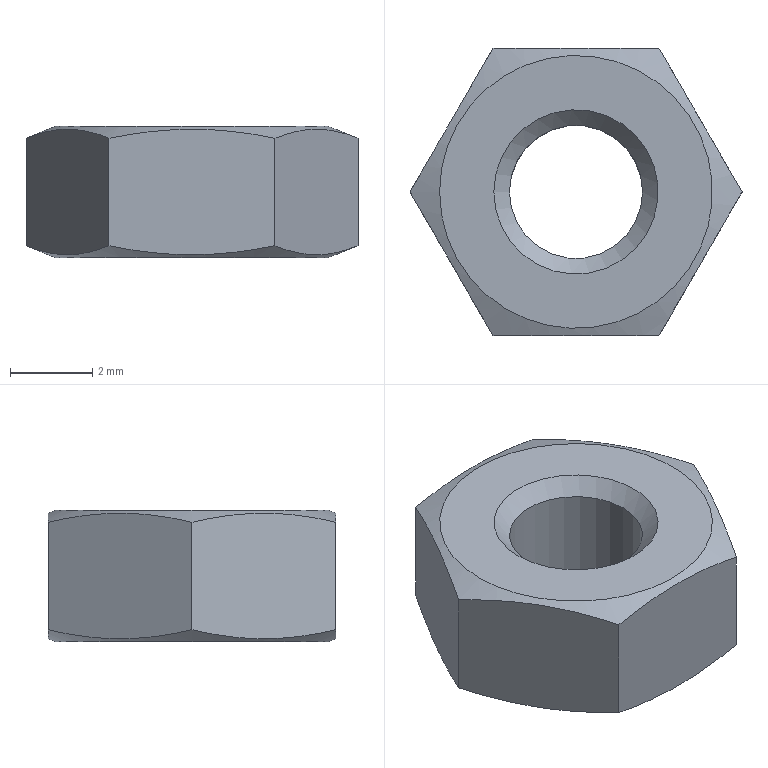Part | STEP file | 1_33 | 1 solid | 13 faces | box 8.083 x 7 x 3.2 mm | volume 106.427 mm3 | plane 8 | cone 4 | cylinder 1 | commonest cylinder face diameters 3.242 x1
STEP:
#1=CARTESIAN_POINT('',(0.,0.,0.));
#2=DIRECTION('',(0.,0.,1.));
#3=DIRECTION('',(1.,0.,0.));
#4=AXIS2_PLACEMENT_3D('',#1,#2,#3);
#5=CARTESIAN_POINT('',(-1.621,0.,0.3789));
#6=VERTEX_POINT('',#5);
#7=CARTESIAN_POINT('',(0.,0.,0.3789));
#8=DIRECTION('',(0.,0.,-1.));
#9=DIRECTION('',(1.,0.,0.));
#10=AXIS2_PLACEMENT_3D('',#7,#8,#9);
#11=CIRCLE('',#10,1.621);
#12=CARTESIAN_POINT('',(0.,0.,0.1894));
#13=DIRECTION('',(0.,0.,-1.));
#14=DIRECTION('',(1.,0.,0.));
#15=AXIS2_PLACEMENT_3D('',#12,#13,#14);
#16=CONICAL_SURFACE('',#15,1.811,0.7854);
#17=CARTESIAN_POINT('',(0.,-0.1894));
#18=DIRECTION('',(1.,0.));
#19=VECTOR('',#18,1.);
#20=LINE('',#17,#19);
#21=(GEOMETRIC_REPRESENTATION_CONTEXT(2)PARAMETRIC_REPRESENTATION_CONTEXT()REPRESENTATION_CONTEXT('',''));
#22=DEFINITIONAL_REPRESENTATION('',(#20),#21);
#23=PCURVE('',#16,#22);
#24=CARTESIAN_POINT('',(0.,0.,1.6));
#25=DIRECTION('',(0.,0.,-1.));
#26=DIRECTION('',(1.,0.,0.));
#27=AXIS2_PLACEMENT_3D('',#24,#25,#26);
#28=CYLINDRICAL_SURFACE('',#27,1.621);
#29=CARTESIAN_POINT('',(0.,1.221));
#30=DIRECTION('',(1.,0.));
#31=VECTOR('',#30,1.);
#32=LINE('',#29,#31);
#33=(GEOMETRIC_REPRESENTATION_CONTEXT(2)PARAMETRIC_REPRESENTATION_CONTEXT()REPRESENTATION_CONTEXT('',''));
#34=DEFINITIONAL_REPRESENTATION('',(#32),#33);
#35=PCURVE('',#28,#34);
#36=SURFACE_CURVE('',#11,(#23,#35),.PCURVE_S1.);
#37=EDGE_CURVE('',#6,#6,#36,.T.);
#38=ORIENTED_EDGE('',*,*,#37,.T.);
#39=CARTESIAN_POINT('',(-2.,0.,0.));
#40=VERTEX_POINT('',#39);
#41=CARTESIAN_POINT('',(-1.621,0.,0.3789));
#42=CARTESIAN_POINT('',(-2.,0.,0.));
#43=B_SPLINE_CURVE_WITH_KNOTS('',1,(#41,#42),.UNSPECIFIED.,.F.,.F.,(2,2),(-0.2679,0.2679),.PIECEWISE_BEZIER_KNOTS.);
#44=CARTESIAN_POINT('',(9.425,0.));
#45=DIRECTION('',(0.,1.));
#46=VECTOR('',#45,1.);
#47=LINE('',#44,#46);
#48=(GEOMETRIC_REPRESENTATION_CONTEXT(2)PARAMETRIC_REPRESENTATION_CONTEXT()REPRESENTATION_CONTEXT('',''));
#49=DEFINITIONAL_REPRESENTATION('',(#47),#48);
#50=PCURVE('',#16,#49);
#51=CARTESIAN_POINT('',(3.142,0.));
#52=DIRECTION('',(0.,1.));
#53=VECTOR('',#52,1.);
#54=LINE('',#51,#53);
#55=(GEOMETRIC_REPRESENTATION_CONTEXT(2)PARAMETRIC_REPRESENTATION_CONTEXT()REPRESENTATION_CONTEXT('',''));
#56=DEFINITIONAL_REPRESENTATION('',(#54),#55);
#57=PCURVE('',#16,#56);
#58=SEAM_CURVE('',#43,(#50,#57),.PCURVE_S1.);
#59=EDGE_CURVE('',#6,#40,#58,.T.);
#60=ORIENTED_EDGE('',*,*,#59,.T.);
#61=CARTESIAN_POINT('',(0.,0.,0.));
#62=DIRECTION('',(0.,0.,-1.));
#63=DIRECTION('',(1.,0.,0.));
#64=AXIS2_PLACEMENT_3D('',#61,#62,#63);
#65=CIRCLE('',#64,2.);
#66=CARTESIAN_POINT('',(0.,0.1894));
#67=DIRECTION('',(1.,0.));
#68=VECTOR('',#67,1.);
#69=LINE('',#66,#68);
#70=(GEOMETRIC_REPRESENTATION_CONTEXT(2)PARAMETRIC_REPRESENTATION_CONTEXT()REPRESENTATION_CONTEXT('',''));
#71=DEFINITIONAL_REPRESENTATION('',(#69),#70);
#72=PCURVE('',#16,#71);
#73=CARTESIAN_POINT('',(0.,0.,0.));
#74=DIRECTION('',(0.,0.,1.));
#75=DIRECTION('',(1.,0.,0.));
#76=AXIS2_PLACEMENT_3D('',#73,#74,#75);
#77=PLANE('',#76);
#78=CARTESIAN_POINT('',(2.,0.));
#79=CARTESIAN_POINT('',(2.,-3.464));
#80=CARTESIAN_POINT('',(-1.,-1.732));
#81=CARTESIAN_POINT('',(-4.,0.));
#82=CARTESIAN_POINT('',(-1.,1.732));
#83=CARTESIAN_POINT('',(2.,3.464));
#84=CARTESIAN_POINT('',(2.,0.));
#85=(BOUNDED_CURVE()B_SPLINE_CURVE(2,(#78,#79,#80,#81,#82,#83,#84),.UNSPECIFIED.,.T.,.F.)B_SPLINE_CURVE_WITH_KNOTS((1,2,2,2,2,1),(-2.094,0.,2.094,4.189,6.283,8.378),.UNSPECIFIED.)CURVE()GEOMETRIC_REPRESENTATION_ITEM()RATIONAL_B_SPLINE_CURVE((1.,0.5,1.,0.5,1.,0.5,1.))REPRESENTATION_ITEM(''));
#86=(GEOMETRIC_REPRESENTATION_CONTEXT(2)PARAMETRIC_REPRESENTATION_CONTEXT()REPRESENTATION_CONTEXT('',''));
#87=DEFINITIONAL_REPRESENTATION('',(#85),#86);
#88=PCURVE('',#77,#87);
#89=SURFACE_CURVE('',#65,(#72,#88),.PCURVE_S1.);
#90=EDGE_CURVE('',#40,#40,#89,.T.);
#91=ORIENTED_EDGE('',*,*,#90,.F.);
#92=ORIENTED_EDGE('',*,*,#59,.F.);
#93=EDGE_LOOP('',(#38,#60,#91,#92));
#94=FACE_BOUND('',#93,.F.);
#95=ADVANCED_FACE('',(#94),#16,.F.);
#96=CARTESIAN_POINT('',(-3.321,0.,0.));
#97=VERTEX_POINT('',#96);
#98=CARTESIAN_POINT('',(0.,0.,0.));
#99=DIRECTION('',(0.,0.,1.));
#100=DIRECTION('',(1.,0.,0.));
#101=AXIS2_PLACEMENT_3D('',#98,#99,#100);
#102=CIRCLE('',#101,3.321);
#103=CARTESIAN_POINT('',(0.,0.));
#104=DIRECTION('',(1.,0.));
#105=AXIS2_PLACEMENT_2D('',#103,#104);
#106=CIRCLE('',#105,3.321);
#107=(GEOMETRIC_REPRESENTATION_CONTEXT(2)PARAMETRIC_REPRESENTATION_CONTEXT()REPRESENTATION_CONTEXT('',''));
#108=DEFINITIONAL_REPRESENTATION('',(#106),#107);
#109=PCURVE('',#77,#108);
#110=CARTESIAN_POINT('',(0.,0.,0.1455));
#111=DIRECTION('',(0.,0.,1.));
#112=DIRECTION('',(1.,0.,0.));
#113=AXIS2_PLACEMENT_3D('',#110,#111,#112);
#114=CONICAL_SURFACE('',#113,3.681,1.187);
#115=CARTESIAN_POINT('',(0.,-0.1455));
#116=DIRECTION('',(1.,0.));
#117=VECTOR('',#116,1.);
#118=LINE('',#115,#117);
#119=(GEOMETRIC_REPRESENTATION_CONTEXT(2)PARAMETRIC_REPRESENTATION_CONTEXT()REPRESENTATION_CONTEXT('',''));
#120=DEFINITIONAL_REPRESENTATION('',(#118),#119);
#121=PCURVE('',#114,#120);
#122=SURFACE_CURVE('',#102,(#109,#121),.PCURVE_S1.);
#123=EDGE_CURVE('',#97,#97,#122,.T.);
#124=ORIENTED_EDGE('',*,*,#123,.F.);
#125=EDGE_LOOP('',(#124));
#126=FACE_BOUND('',#125,.T.);
#127=ORIENTED_EDGE('',*,*,#90,.F.);
#128=EDGE_LOOP('',(#127));
#129=FACE_BOUND('',#128,.T.);
#130=ADVANCED_FACE('',(#126,#129),#77,.F.);
#131=CARTESIAN_POINT('',(-1.621,0.,2.821));
#132=VERTEX_POINT('',#131);
#133=CARTESIAN_POINT('',(0.,0.,2.821));
#134=DIRECTION('',(0.,0.,-1.));
#135=DIRECTION('',(1.,0.,0.));
#136=AXIS2_PLACEMENT_3D('',#133,#134,#135);
#137=CIRCLE('',#136,1.621);
#138=CARTESIAN_POINT('',(0.,-1.221));
#139=DIRECTION('',(1.,0.));
#140=VECTOR('',#139,1.);
#141=LINE('',#138,#140);
#142=(GEOMETRIC_REPRESENTATION_CONTEXT(2)PARAMETRIC_REPRESENTATION_CONTEXT()REPRESENTATION_CONTEXT('',''));
#143=DEFINITIONAL_REPRESENTATION('',(#141),#142);
#144=PCURVE('',#28,#143);
#145=CARTESIAN_POINT('',(0.,0.,3.011));
#146=DIRECTION('',(0.,0.,1.));
#147=DIRECTION('',(-1.,0.,0.));
#148=AXIS2_PLACEMENT_3D('',#145,#146,#147);
#149=CONICAL_SURFACE('',#148,1.811,0.7854);
#150=CARTESIAN_POINT('',(9.425,-0.1894));
#151=DIRECTION('',(-1.,0.));
#152=VECTOR('',#151,1.);
#153=LINE('',#150,#152);
#154=(GEOMETRIC_REPRESENTATION_CONTEXT(2)PARAMETRIC_REPRESENTATION_CONTEXT()REPRESENTATION_CONTEXT('',''));
#155=DEFINITIONAL_REPRESENTATION('',(#153),#154);
#156=PCURVE('',#149,#155);
#157=SURFACE_CURVE('',#137,(#144,#156),.PCURVE_S1.);
#158=EDGE_CURVE('',#132,#132,#157,.T.);
#159=ORIENTED_EDGE('',*,*,#158,.T.);
#160=CARTESIAN_POINT('',(-1.621,0.,2.821));
#161=CARTESIAN_POINT('',(-1.621,0.,0.3789));
#162=B_SPLINE_CURVE_WITH_KNOTS('',1,(#160,#161),.UNSPECIFIED.,.F.,.F.,(2,2),(-1.221,1.221),.PIECEWISE_BEZIER_KNOTS.);
#163=CARTESIAN_POINT('',(9.425,0.));
#164=DIRECTION('',(0.,1.));
#165=VECTOR('',#164,1.);
#166=LINE('',#163,#165);
#167=(GEOMETRIC_REPRESENTATION_CONTEXT(2)PARAMETRIC_REPRESENTATION_CONTEXT()REPRESENTATION_CONTEXT('',''));
#168=DEFINITIONAL_REPRESENTATION('',(#166),#167);
#169=PCURVE('',#28,#168);
#170=CARTESIAN_POINT('',(3.142,0.));
#171=DIRECTION('',(0.,1.));
#172=VECTOR('',#171,1.);
#173=LINE('',#170,#172);
#174=(GEOMETRIC_REPRESENTATION_CONTEXT(2)PARAMETRIC_REPRESENTATION_CONTEXT()REPRESENTATION_CONTEXT('',''));
#175=DEFINITIONAL_REPRESENTATION('',(#173),#174);
#176=PCURVE('',#28,#175);
#177=SEAM_CURVE('',#162,(#169,#176),.PCURVE_S1.);
#178=EDGE_CURVE('',#132,#6,#177,.T.);
#179=ORIENTED_EDGE('',*,*,#178,.T.);
#180=ORIENTED_EDGE('',*,*,#37,.F.);
#181=ORIENTED_EDGE('',*,*,#178,.F.);
#182=EDGE_LOOP('',(#159,#179,#180,#181));
#183=FACE_BOUND('',#182,.F.);
#184=ADVANCED_FACE('',(#183),#28,.F.);
#185=CARTESIAN_POINT('',(-4.041,0.,0.2909));
#186=VERTEX_POINT('',#185);
#187=CARTESIAN_POINT('',(-2.021,3.5,0.2909));
#188=VERTEX_POINT('',#187);
#189=CARTESIAN_POINT('',(-9.627,-9.674,4.172));
#190=CARTESIAN_POINT('',(-3.031,1.75,-0.9793));
#191=CARTESIAN_POINT('',(3.564,13.174,4.172));
#192=(BOUNDED_CURVE()B_SPLINE_CURVE(2,(#189,#190,#191),.UNSPECIFIED.,.F.,.F.)B_SPLINE_CURVE_WITH_KNOTS((3,3),(0.,2.763),.PIECEWISE_BEZIER_KNOTS.)CURVE()GEOMETRIC_REPRESENTATION_ITEM()RATIONAL_B_SPLINE_CURVE((1.,3.899,1.))REPRESENTATION_ITEM(''));
#193=CARTESIAN_POINT('',(9.425,0.1455));
#194=CARTESIAN_POINT('',(9.41,0.1312));
#195=CARTESIAN_POINT('',(9.379,0.1043));
#196=CARTESIAN_POINT('',(9.333,0.06874));
#197=CARTESIAN_POINT('',(9.286,0.03763));
#198=CARTESIAN_POINT('',(9.239,0.01072));
#199=CARTESIAN_POINT('',(9.191,-0.01221));
#200=CARTESIAN_POINT('',(9.144,-0.03133));
#201=CARTESIAN_POINT('',(9.095,-0.04679));
#202=CARTESIAN_POINT('',(9.047,-0.0587));
#203=CARTESIAN_POINT('',(8.999,-0.06714));
#204=CARTESIAN_POINT('',(8.95,-0.07219));
#205=CARTESIAN_POINT('',(8.901,-0.07387));
#206=CARTESIAN_POINT('',(8.852,-0.07219));
#207=CARTESIAN_POINT('',(8.804,-0.06714));
#208=CARTESIAN_POINT('',(8.755,-0.0587));
#209=CARTESIAN_POINT('',(8.707,-0.04679));
#210=CARTESIAN_POINT('',(8.659,-0.03133));
#211=CARTESIAN_POINT('',(8.611,-0.01221));
#212=CARTESIAN_POINT('',(8.563,0.01072));
#213=CARTESIAN_POINT('',(8.516,0.03763));
#214=CARTESIAN_POINT('',(8.469,0.06874));
#215=CARTESIAN_POINT('',(8.423,0.1043));
#216=CARTESIAN_POINT('',(8.393,0.1312));
#217=CARTESIAN_POINT('',(8.378,0.1455));
#218=B_SPLINE_CURVE_WITH_KNOTS('',3,(#193,#194,#195,#196,#197,#198,#199,#200,#201,#202,#203,#204,#205,#206,#207,#208,#209,#210,#211,#212,#213,#214,#215,#216,#217),.UNSPECIFIED.,.F.,.F.,(4,1,1,1,1,1,1,1,1,1,1,1,1,1,1,1,1,1,1,1,1,1,4),(0.9002,0.9439,0.9877,1.031,1.075,1.119,1.163,1.206,1.25,1.294,1.338,1.381,1.425,1.469,1.513,1.556,1.6,1.644,1.688,1.731,1.775,1.819,1.863),.QUASI_UNIFORM_KNOTS.);
#219=(GEOMETRIC_REPRESENTATION_CONTEXT(2)PARAMETRIC_REPRESENTATION_CONTEXT()REPRESENTATION_CONTEXT('',''));
#220=DEFINITIONAL_REPRESENTATION('',(#218),#219);
#221=PCURVE('',#114,#220);
#222=CARTESIAN_POINT('',(-4.041,0.,0.));
#223=DIRECTION('',(-0.866,0.5,0.));
#224=DIRECTION('',(0.,0.,1.));
#225=AXIS2_PLACEMENT_3D('',#222,#223,#224);
#226=PLANE('',#225);
#227=CARTESIAN_POINT('',(4.172,-11.17));
#228=CARTESIAN_POINT('',(-0.9793,2.021));
#229=CARTESIAN_POINT('',(4.172,15.212));
#230=(BOUNDED_CURVE()B_SPLINE_CURVE(2,(#227,#228,#229),.UNSPECIFIED.,.F.,.F.)B_SPLINE_CURVE_WITH_KNOTS((3,3),(0.,2.763),.PIECEWISE_BEZIER_KNOTS.)CURVE()GEOMETRIC_REPRESENTATION_ITEM()RATIONAL_B_SPLINE_CURVE((1.,3.899,1.))REPRESENTATION_ITEM(''));
#231=(GEOMETRIC_REPRESENTATION_CONTEXT(2)PARAMETRIC_REPRESENTATION_CONTEXT()REPRESENTATION_CONTEXT('',''));
#232=DEFINITIONAL_REPRESENTATION('',(#230),#231);
#233=PCURVE('',#226,#232);
#234=SURFACE_CURVE('',#192,(#221,#233),.PCURVE_S1.);
#235=EDGE_CURVE('',#186,#188,#234,.T.);
#236=ORIENTED_EDGE('',*,*,#235,.T.);
#237=CARTESIAN_POINT('',(2.021,3.5,0.2909));
#238=VERTEX_POINT('',#237);
#239=CARTESIAN_POINT('',(-13.191,3.5,4.172));
#240=CARTESIAN_POINT('',(0.,3.5,-0.9793));
#241=CARTESIAN_POINT('',(13.191,3.5,4.172));
#242=(BOUNDED_CURVE()B_SPLINE_CURVE(2,(#239,#240,#241),.UNSPECIFIED.,.F.,.F.)B_SPLINE_CURVE_WITH_KNOTS((3,3),(0.,2.763),.PIECEWISE_BEZIER_KNOTS.)CURVE()GEOMETRIC_REPRESENTATION_ITEM()RATIONAL_B_SPLINE_CURVE((1.,3.899,1.))REPRESENTATION_ITEM(''));
#243=CARTESIAN_POINT('',(8.378,0.1455));
#244=CARTESIAN_POINT('',(8.362,0.1312));
#245=CARTESIAN_POINT('',(8.332,0.1043));
#246=CARTESIAN_POINT('',(8.286,0.06874));
#247=CARTESIAN_POINT('',(8.239,0.03763));
#248=CARTESIAN_POINT('',(8.192,0.01072));
#249=CARTESIAN_POINT('',(8.144,-0.01221));
#250=CARTESIAN_POINT('',(8.096,-0.03133));
#251=CARTESIAN_POINT('',(8.048,-0.04679));
#252=CARTESIAN_POINT('',(8.,-0.0587));
#253=CARTESIAN_POINT('',(7.951,-0.06714));
#254=CARTESIAN_POINT('',(7.903,-0.07219));
#255=CARTESIAN_POINT('',(7.854,-0.07387));
#256=CARTESIAN_POINT('',(7.805,-0.07219));
#257=CARTESIAN_POINT('',(7.757,-0.06714));
#258=CARTESIAN_POINT('',(7.708,-0.0587));
#259=CARTESIAN_POINT('',(7.66,-0.04679));
#260=CARTESIAN_POINT('',(7.612,-0.03133));
#261=CARTESIAN_POINT('',(7.564,-0.01221));
#262=CARTESIAN_POINT('',(7.516,0.01072));
#263=CARTESIAN_POINT('',(7.469,0.03763));
#264=CARTESIAN_POINT('',(7.422,0.06874));
#265=CARTESIAN_POINT('',(7.376,0.1043));
#266=CARTESIAN_POINT('',(7.346,0.1312));
#267=CARTESIAN_POINT('',(7.33,0.1455));
#268=B_SPLINE_CURVE_WITH_KNOTS('',3,(#243,#244,#245,#246,#247,#248,#249,#250,#251,#252,#253,#254,#255,#256,#257,#258,#259,#260,#261,#262,#263,#264,#265,#266,#267),.UNSPECIFIED.,.F.,.F.,(4,1,1,1,1,1,1,1,1,1,1,1,1,1,1,1,1,1,1,1,1,1,4),(0.9002,0.9439,0.9877,1.031,1.075,1.119,1.163,1.206,1.25,1.294,1.338,1.381,1.425,1.469,1.513,1.556,1.6,1.644,1.688,1.731,1.775,1.819,1.863),.QUASI_UNIFORM_KNOTS.);
#269=(GEOMETRIC_REPRESENTATION_CONTEXT(2)PARAMETRIC_REPRESENTATION_CONTEXT()REPRESENTATION_CONTEXT('',''));
#270=DEFINITIONAL_REPRESENTATION('',(#268),#269);
#271=PCURVE('',#114,#270);
#272=CARTESIAN_POINT('',(-2.021,3.5,0.));
#273=DIRECTION('',(0.,1.,0.));
#274=DIRECTION('',(0.,0.,1.));
#275=AXIS2_PLACEMENT_3D('',#272,#273,#274);
#276=PLANE('',#275);
#277=CARTESIAN_POINT('',(4.172,-11.17));
#278=CARTESIAN_POINT('',(-0.9793,2.021));
#279=CARTESIAN_POINT('',(4.172,15.212));
#280=(BOUNDED_CURVE()B_SPLINE_CURVE(2,(#277,#278,#279),.UNSPECIFIED.,.F.,.F.)B_SPLINE_CURVE_WITH_KNOTS((3,3),(0.,2.763),.PIECEWISE_BEZIER_KNOTS.)CURVE()GEOMETRIC_REPRESENTATION_ITEM()RATIONAL_B_SPLINE_CURVE((1.,3.899,1.))REPRESENTATION_ITEM(''));
#281=(GEOMETRIC_REPRESENTATION_CONTEXT(2)PARAMETRIC_REPRESENTATION_CONTEXT()REPRESENTATION_CONTEXT('',''));
#282=DEFINITIONAL_REPRESENTATION('',(#280),#281);
#283=PCURVE('',#276,#282);
#284=SURFACE_CURVE('',#242,(#271,#283),.PCURVE_S1.);
#285=EDGE_CURVE('',#188,#238,#284,.T.);
#286=ORIENTED_EDGE('',*,*,#285,.T.);
#287=CARTESIAN_POINT('',(4.041,0.,0.2909));
#288=VERTEX_POINT('',#287);
#289=CARTESIAN_POINT('',(-3.564,13.174,4.172));
#290=CARTESIAN_POINT('',(3.031,1.75,-0.9793));
#291=CARTESIAN_POINT('',(9.627,-9.674,4.172));
#292=(BOUNDED_CURVE()B_SPLINE_CURVE(2,(#289,#290,#291),.UNSPECIFIED.,.F.,.F.)B_SPLINE_CURVE_WITH_KNOTS((3,3),(0.,2.763),.PIECEWISE_BEZIER_KNOTS.)CURVE()GEOMETRIC_REPRESENTATION_ITEM()RATIONAL_B_SPLINE_CURVE((1.,3.899,1.))REPRESENTATION_ITEM(''));
#293=CARTESIAN_POINT('',(7.33,0.1455));
#294=CARTESIAN_POINT('',(7.315,0.1312));
#295=CARTESIAN_POINT('',(7.285,0.1043));
#296=CARTESIAN_POINT('',(7.238,0.06874));
#297=CARTESIAN_POINT('',(7.192,0.03763));
#298=CARTESIAN_POINT('',(7.145,0.01072));
#299=CARTESIAN_POINT('',(7.097,-0.01221));
#300=CARTESIAN_POINT('',(7.049,-0.03133));
#301=CARTESIAN_POINT('',(7.001,-0.04679));
#302=CARTESIAN_POINT('',(6.953,-0.0587));
#303=CARTESIAN_POINT('',(6.904,-0.06714));
#304=CARTESIAN_POINT('',(6.856,-0.07219));
#305=CARTESIAN_POINT('',(6.807,-0.07387));
#306=CARTESIAN_POINT('',(6.758,-0.07219));
#307=CARTESIAN_POINT('',(6.709,-0.06714));
#308=CARTESIAN_POINT('',(6.661,-0.0587));
#309=CARTESIAN_POINT('',(6.612,-0.04679));
#310=CARTESIAN_POINT('',(6.564,-0.03133));
#311=CARTESIAN_POINT('',(6.516,-0.01221));
#312=CARTESIAN_POINT('',(6.469,0.01072));
#313=CARTESIAN_POINT('',(6.422,0.03763));
#314=CARTESIAN_POINT('',(6.375,0.06874));
#315=CARTESIAN_POINT('',(6.329,0.1043));
#316=CARTESIAN_POINT('',(6.298,0.1312));
#317=CARTESIAN_POINT('',(6.283,0.1455));
#318=B_SPLINE_CURVE_WITH_KNOTS('',3,(#293,#294,#295,#296,#297,#298,#299,#300,#301,#302,#303,#304,#305,#306,#307,#308,#309,#310,#311,#312,#313,#314,#315,#316,#317),.UNSPECIFIED.,.F.,.F.,(4,1,1,1,1,1,1,1,1,1,1,1,1,1,1,1,1,1,1,1,1,1,4),(0.9002,0.9439,0.9877,1.031,1.075,1.119,1.163,1.206,1.25,1.294,1.338,1.381,1.425,1.469,1.513,1.556,1.6,1.644,1.688,1.731,1.775,1.819,1.863),.QUASI_UNIFORM_KNOTS.);
#319=(GEOMETRIC_REPRESENTATION_CONTEXT(2)PARAMETRIC_REPRESENTATION_CONTEXT()REPRESENTATION_CONTEXT('',''));
#320=DEFINITIONAL_REPRESENTATION('',(#318),#319);
#321=PCURVE('',#114,#320);
#322=CARTESIAN_POINT('',(2.021,3.5,0.));
#323=DIRECTION('',(0.866,0.5,0.));
#324=DIRECTION('',(0.,0.,-1.));
#325=AXIS2_PLACEMENT_3D('',#322,#323,#324);
#326=PLANE('',#325);
#327=CARTESIAN_POINT('',(-4.172,11.17));
#328=CARTESIAN_POINT('',(0.9793,-2.021));
#329=CARTESIAN_POINT('',(-4.172,-15.212));
#330=(BOUNDED_CURVE()B_SPLINE_CURVE(2,(#327,#328,#329),.UNSPECIFIED.,.F.,.F.)B_SPLINE_CURVE_WITH_KNOTS((3,3),(0.,2.763),.PIECEWISE_BEZIER_KNOTS.)CURVE()GEOMETRIC_REPRESENTATION_ITEM()RATIONAL_B_SPLINE_CURVE((1.,3.899,1.))REPRESENTATION_ITEM(''));
#331=(GEOMETRIC_REPRESENTATION_CONTEXT(2)PARAMETRIC_REPRESENTATION_CONTEXT()REPRESENTATION_CONTEXT('',''));
#332=DEFINITIONAL_REPRESENTATION('',(#330),#331);
#333=PCURVE('',#326,#332);
#334=SURFACE_CURVE('',#292,(#321,#333),.PCURVE_S1.);
#335=EDGE_CURVE('',#238,#288,#334,.T.);
#336=ORIENTED_EDGE('',*,*,#335,.T.);
#337=CARTESIAN_POINT('',(2.021,-3.5,0.2909));
#338=VERTEX_POINT('',#337);
#339=CARTESIAN_POINT('',(9.627,9.674,4.172));
#340=CARTESIAN_POINT('',(3.031,-1.75,-0.9793));
#341=CARTESIAN_POINT('',(-3.564,-13.174,4.172));
#342=(BOUNDED_CURVE()B_SPLINE_CURVE(2,(#339,#340,#341),.UNSPECIFIED.,.F.,.F.)B_SPLINE_CURVE_WITH_KNOTS((3,3),(0.,2.763),.PIECEWISE_BEZIER_KNOTS.)CURVE()GEOMETRIC_REPRESENTATION_ITEM()RATIONAL_B_SPLINE_CURVE((1.,3.899,1.))REPRESENTATION_ITEM(''));
#343=CARTESIAN_POINT('',(6.283,0.1455));
#344=CARTESIAN_POINT('',(6.268,0.1312));
#345=CARTESIAN_POINT('',(6.238,0.1043));
#346=CARTESIAN_POINT('',(6.191,0.06874));
#347=CARTESIAN_POINT('',(6.145,0.03763));
#348=CARTESIAN_POINT('',(6.097,0.01072));
#349=CARTESIAN_POINT('',(6.05,-0.01221));
#350=CARTESIAN_POINT('',(6.002,-0.03133));
#351=CARTESIAN_POINT('',(5.954,-0.04679));
#352=CARTESIAN_POINT('',(5.906,-0.0587));
#353=CARTESIAN_POINT('',(5.857,-0.06714));
#354=CARTESIAN_POINT('',(5.808,-0.07219));
#355=CARTESIAN_POINT('',(5.76,-0.07387));
#356=CARTESIAN_POINT('',(5.711,-0.07219));
#357=CARTESIAN_POINT('',(5.662,-0.06714));
#358=CARTESIAN_POINT('',(5.614,-0.0587));
#359=CARTESIAN_POINT('',(5.565,-0.04679));
#360=CARTESIAN_POINT('',(5.517,-0.03133));
#361=CARTESIAN_POINT('',(5.469,-0.01221));
#362=CARTESIAN_POINT('',(5.422,0.01072));
#363=CARTESIAN_POINT('',(5.375,0.03763));
#364=CARTESIAN_POINT('',(5.328,0.06874));
#365=CARTESIAN_POINT('',(5.282,0.1043));
#366=CARTESIAN_POINT('',(5.251,0.1312));
#367=CARTESIAN_POINT('',(5.236,0.1455));
#368=B_SPLINE_CURVE_WITH_KNOTS('',3,(#343,#344,#345,#346,#347,#348,#349,#350,#351,#352,#353,#354,#355,#356,#357,#358,#359,#360,#361,#362,#363,#364,#365,#366,#367),.UNSPECIFIED.,.F.,.F.,(4,1,1,1,1,1,1,1,1,1,1,1,1,1,1,1,1,1,1,1,1,1,4),(0.9002,0.9439,0.9877,1.031,1.075,1.119,1.163,1.206,1.25,1.294,1.338,1.381,1.425,1.469,1.513,1.556,1.6,1.644,1.688,1.731,1.775,1.819,1.863),.QUASI_UNIFORM_KNOTS.);
#369=(GEOMETRIC_REPRESENTATION_CONTEXT(2)PARAMETRIC_REPRESENTATION_CONTEXT()REPRESENTATION_CONTEXT('',''));
#370=DEFINITIONAL_REPRESENTATION('',(#368),#369);
#371=PCURVE('',#114,#370);
#372=CARTESIAN_POINT('',(4.041,0.,0.));
#373=DIRECTION('',(0.866,-0.5,0.));
#374=DIRECTION('',(0.,0.,-1.));
#375=AXIS2_PLACEMENT_3D('',#372,#373,#374);
#376=PLANE('',#375);
#377=CARTESIAN_POINT('',(-4.172,11.17));
#378=CARTESIAN_POINT('',(0.9793,-2.021));
#379=CARTESIAN_POINT('',(-4.172,-15.212));
#380=(BOUNDED_CURVE()B_SPLINE_CURVE(2,(#377,#378,#379),.UNSPECIFIED.,.F.,.F.)B_SPLINE_CURVE_WITH_KNOTS((3,3),(0.,2.763),.PIECEWISE_BEZIER_KNOTS.)CURVE()GEOMETRIC_REPRESENTATION_ITEM()RATIONAL_B_SPLINE_CURVE((1.,3.899,1.))REPRESENTATION_ITEM(''));
#381=(GEOMETRIC_REPRESENTATION_CONTEXT(2)PARAMETRIC_REPRESENTATION_CONTEXT()REPRESENTATION_CONTEXT('',''));
#382=DEFINITIONAL_REPRESENTATION('',(#380),#381);
#383=PCURVE('',#376,#382);
#384=SURFACE_CURVE('',#342,(#371,#383),.PCURVE_S1.);
#385=EDGE_CURVE('',#288,#338,#384,.T.);
#386=ORIENTED_EDGE('',*,*,#385,.T.);
#387=CARTESIAN_POINT('',(-2.021,-3.5,0.2909));
#388=VERTEX_POINT('',#387);
#389=CARTESIAN_POINT('',(13.191,-3.5,4.172));
#390=CARTESIAN_POINT('',(0.,-3.5,-0.9793));
#391=CARTESIAN_POINT('',(-13.191,-3.5,4.172));
#392=(BOUNDED_CURVE()B_SPLINE_CURVE(2,(#389,#390,#391),.UNSPECIFIED.,.F.,.F.)B_SPLINE_CURVE_WITH_KNOTS((3,3),(0.,2.763),.PIECEWISE_BEZIER_KNOTS.)CURVE()GEOMETRIC_REPRESENTATION_ITEM()RATIONAL_B_SPLINE_CURVE((1.,3.899,1.))REPRESENTATION_ITEM(''));
#393=CARTESIAN_POINT('',(5.236,0.1455));
#394=CARTESIAN_POINT('',(5.221,0.1312));
#395=CARTESIAN_POINT('',(5.19,0.1043));
#396=CARTESIAN_POINT('',(5.144,0.06874));
#397=CARTESIAN_POINT('',(5.097,0.03763));
#398=CARTESIAN_POINT('',(5.05,0.01072));
#399=CARTESIAN_POINT('',(5.003,-0.01221));
#400=CARTESIAN_POINT('',(4.955,-0.03133));
#401=CARTESIAN_POINT('',(4.907,-0.04679));
#402=CARTESIAN_POINT('',(4.858,-0.0587));
#403=CARTESIAN_POINT('',(4.81,-0.06714));
#404=CARTESIAN_POINT('',(4.761,-0.07219));
#405=CARTESIAN_POINT('',(4.712,-0.07387));
#406=CARTESIAN_POINT('',(4.664,-0.07219));
#407=CARTESIAN_POINT('',(4.615,-0.06714));
#408=CARTESIAN_POINT('',(4.566,-0.0587));
#409=CARTESIAN_POINT('',(4.518,-0.04679));
#410=CARTESIAN_POINT('',(4.47,-0.03133));
#411=CARTESIAN_POINT('',(4.422,-0.01221));
#412=CARTESIAN_POINT('',(4.375,0.01072));
#413=CARTESIAN_POINT('',(4.327,0.03763));
#414=CARTESIAN_POINT('',(4.281,0.06874));
#415=CARTESIAN_POINT('',(4.234,0.1043));
#416=CARTESIAN_POINT('',(4.204,0.1312));
#417=CARTESIAN_POINT('',(4.189,0.1455));
#418=B_SPLINE_CURVE_WITH_KNOTS('',3,(#393,#394,#395,#396,#397,#398,#399,#400,#401,#402,#403,#404,#405,#406,#407,#408,#409,#410,#411,#412,#413,#414,#415,#416,#417),.UNSPECIFIED.,.F.,.F.,(4,1,1,1,1,1,1,1,1,1,1,1,1,1,1,1,1,1,1,1,1,1,4),(0.9002,0.9439,0.9877,1.031,1.075,1.119,1.163,1.206,1.25,1.294,1.338,1.381,1.425,1.469,1.513,1.556,1.6,1.644,1.688,1.731,1.775,1.819,1.863),.QUASI_UNIFORM_KNOTS.);
#419=(GEOMETRIC_REPRESENTATION_CONTEXT(2)PARAMETRIC_REPRESENTATION_CONTEXT()REPRESENTATION_CONTEXT('',''));
#420=DEFINITIONAL_REPRESENTATION('',(#418),#419);
#421=PCURVE('',#114,#420);
#422=CARTESIAN_POINT('',(2.021,-3.5,0.));
#423=DIRECTION('',(0.,-1.,0.));
#424=DIRECTION('',(0.,0.,-1.));
#425=AXIS2_PLACEMENT_3D('',#422,#423,#424);
#426=PLANE('',#425);
#427=CARTESIAN_POINT('',(-4.172,11.17));
#428=CARTESIAN_POINT('',(0.9793,-2.021));
#429=CARTESIAN_POINT('',(-4.172,-15.212));
#430=(BOUNDED_CURVE()B_SPLINE_CURVE(2,(#427,#428,#429),.UNSPECIFIED.,.F.,.F.)B_SPLINE_CURVE_WITH_KNOTS((3,3),(0.,2.763),.PIECEWISE_BEZIER_KNOTS.)CURVE()GEOMETRIC_REPRESENTATION_ITEM()RATIONAL_B_SPLINE_CURVE((1.,3.899,1.))REPRESENTATION_ITEM(''));
#431=(GEOMETRIC_REPRESENTATION_CONTEXT(2)PARAMETRIC_REPRESENTATION_CONTEXT()REPRESENTATION_CONTEXT('',''));
#432=DEFINITIONAL_REPRESENTATION('',(#430),#431);
#433=PCURVE('',#426,#432);
#434=SURFACE_CURVE('',#392,(#421,#433),.PCURVE_S1.);
#435=EDGE_CURVE('',#338,#388,#434,.T.);
#436=ORIENTED_EDGE('',*,*,#435,.T.);
#437=CARTESIAN_POINT('',(3.564,-13.174,4.172));
#438=CARTESIAN_POINT('',(-3.031,-1.75,-0.9793));
#439=CARTESIAN_POINT('',(-9.627,9.674,4.172));
#440=(BOUNDED_CURVE()B_SPLINE_CURVE(2,(#437,#438,#439),.UNSPECIFIED.,.F.,.F.)B_SPLINE_CURVE_WITH_KNOTS((3,3),(0.,2.763),.PIECEWISE_BEZIER_KNOTS.)CURVE()GEOMETRIC_REPRESENTATION_ITEM()RATIONAL_B_SPLINE_CURVE((1.,3.899,1.))REPRESENTATION_ITEM(''));
#441=CARTESIAN_POINT('',(4.189,0.1455));
#442=CARTESIAN_POINT('',(4.174,0.1312));
#443=CARTESIAN_POINT('',(4.143,0.1043));
#444=CARTESIAN_POINT('',(4.097,0.06874));
#445=CARTESIAN_POINT('',(4.05,0.03763));
#446=CARTESIAN_POINT('',(4.003,0.01072));
#447=CARTESIAN_POINT('',(3.956,-0.01221));
#448=CARTESIAN_POINT('',(3.908,-0.03133));
#449=CARTESIAN_POINT('',(3.859,-0.04679));
#450=CARTESIAN_POINT('',(3.811,-0.0587));
#451=CARTESIAN_POINT('',(3.763,-0.06714));
#452=CARTESIAN_POINT('',(3.714,-0.07219));
#453=CARTESIAN_POINT('',(3.665,-0.07387));
#454=CARTESIAN_POINT('',(3.616,-0.07219));
#455=CARTESIAN_POINT('',(3.568,-0.06714));
#456=CARTESIAN_POINT('',(3.519,-0.0587));
#457=CARTESIAN_POINT('',(3.471,-0.04679));
#458=CARTESIAN_POINT('',(3.423,-0.03133));
#459=CARTESIAN_POINT('',(3.375,-0.01221));
#460=CARTESIAN_POINT('',(3.327,0.01072));
#461=CARTESIAN_POINT('',(3.28,0.03763));
#462=CARTESIAN_POINT('',(3.233,0.06874));
#463=CARTESIAN_POINT('',(3.187,0.1043));
#464=CARTESIAN_POINT('',(3.157,0.1312));
#465=CARTESIAN_POINT('',(3.142,0.1455));
#466=B_SPLINE_CURVE_WITH_KNOTS('',3,(#441,#442,#443,#444,#445,#446,#447,#448,#449,#450,#451,#452,#453,#454,#455,#456,#457,#458,#459,#460,#461,#462,#463,#464,#465),.UNSPECIFIED.,.F.,.F.,(4,1,1,1,1,1,1,1,1,1,1,1,1,1,1,1,1,1,1,1,1,1,4),(0.9002,0.9439,0.9877,1.031,1.075,1.119,1.163,1.206,1.25,1.294,1.338,1.381,1.425,1.469,1.513,1.556,1.6,1.644,1.688,1.731,1.775,1.819,1.863),.QUASI_UNIFORM_KNOTS.);
#467=(GEOMETRIC_REPRESENTATION_CONTEXT(2)PARAMETRIC_REPRESENTATION_CONTEXT()REPRESENTATION_CONTEXT('',''));
#468=DEFINITIONAL_REPRESENTATION('',(#466),#467);
#469=PCURVE('',#114,#468);
#470=CARTESIAN_POINT('',(-2.021,-3.5,0.));
#471=DIRECTION('',(-0.866,-0.5,0.));
#472=DIRECTION('',(0.,0.,1.));
#473=AXIS2_PLACEMENT_3D('',#470,#471,#472);
#474=PLANE('',#473);
#475=CARTESIAN_POINT('',(4.172,-11.17));
#476=CARTESIAN_POINT('',(-0.9793,2.021));
#477=CARTESIAN_POINT('',(4.172,15.212));
#478=(BOUNDED_CURVE()B_SPLINE_CURVE(2,(#475,#476,#477),.UNSPECIFIED.,.F.,.F.)B_SPLINE_CURVE_WITH_KNOTS((3,3),(0.,2.763),.PIECEWISE_BEZIER_KNOTS.)CURVE()GEOMETRIC_REPRESENTATION_ITEM()RATIONAL_B_SPLINE_CURVE((1.,3.899,1.))REPRESENTATION_ITEM(''));
#479=(GEOMETRIC_REPRESENTATION_CONTEXT(2)PARAMETRIC_REPRESENTATION_CONTEXT()REPRESENTATION_CONTEXT('',''));
#480=DEFINITIONAL_REPRESENTATION('',(#478),#479);
#481=PCURVE('',#474,#480);
#482=SURFACE_CURVE('',#440,(#469,#481),.PCURVE_S1.);
#483=EDGE_CURVE('',#388,#186,#482,.T.);
#484=ORIENTED_EDGE('',*,*,#483,.T.);
#485=CARTESIAN_POINT('',(-3.321,0.,0.));
#486=CARTESIAN_POINT('',(-4.041,0.,0.2909));
#487=B_SPLINE_CURVE_WITH_KNOTS('',1,(#485,#486),.UNSPECIFIED.,.F.,.F.,(2,2),(-0.3883,0.3883),.PIECEWISE_BEZIER_KNOTS.);
#488=CARTESIAN_POINT('',(3.142,0.));
#489=DIRECTION('',(0.,1.));
#490=VECTOR('',#489,1.);
#491=LINE('',#488,#490);
#492=(GEOMETRIC_REPRESENTATION_CONTEXT(2)PARAMETRIC_REPRESENTATION_CONTEXT()REPRESENTATION_CONTEXT('',''));
#493=DEFINITIONAL_REPRESENTATION('',(#491),#492);
#494=PCURVE('',#114,#493);
#495=CARTESIAN_POINT('',(9.425,0.));
#496=DIRECTION('',(0.,1.));
#497=VECTOR('',#496,1.);
#498=LINE('',#495,#497);
#499=(GEOMETRIC_REPRESENTATION_CONTEXT(2)PARAMETRIC_REPRESENTATION_CONTEXT()REPRESENTATION_CONTEXT('',''));
#500=DEFINITIONAL_REPRESENTATION('',(#498),#499);
#501=PCURVE('',#114,#500);
#502=SEAM_CURVE('',#487,(#494,#501),.PCURVE_S1.);
#503=EDGE_CURVE('',#97,#186,#502,.T.);
#504=ORIENTED_EDGE('',*,*,#503,.F.);
#505=ORIENTED_EDGE('',*,*,#123,.T.);
#506=ORIENTED_EDGE('',*,*,#503,.T.);
#507=EDGE_LOOP('',(#236,#286,#336,#386,#436,#484,#504,#505,#506));
#508=FACE_BOUND('',#507,.T.);
#509=ADVANCED_FACE('',(#508),#114,.T.);
#510=CARTESIAN_POINT('',(-2.,0.,3.2));
#511=VERTEX_POINT('',#510);
#512=CARTESIAN_POINT('',(0.,0.,3.2));
#513=DIRECTION('',(0.,0.,1.));
#514=DIRECTION('',(1.,0.,0.));
#515=AXIS2_PLACEMENT_3D('',#512,#513,#514);
#516=CIRCLE('',#515,2.);
#517=CARTESIAN_POINT('',(-3.142,0.1894));
#518=DIRECTION('',(1.,0.));
#519=VECTOR('',#518,1.);
#520=LINE('',#517,#519);
#521=(GEOMETRIC_REPRESENTATION_CONTEXT(2)PARAMETRIC_REPRESENTATION_CONTEXT()REPRESENTATION_CONTEXT('',''));
#522=DEFINITIONAL_REPRESENTATION('',(#520),#521);
#523=PCURVE('',#149,#522);
#524=CARTESIAN_POINT('',(0.,0.,3.2));
#525=DIRECTION('',(0.,0.,1.));
#526=DIRECTION('',(1.,0.,0.));
#527=AXIS2_PLACEMENT_3D('',#524,#525,#526);
#528=PLANE('',#527);
#529=CARTESIAN_POINT('',(0.,0.));
#530=DIRECTION('',(1.,0.));
#531=AXIS2_PLACEMENT_2D('',#529,#530);
#532=CIRCLE('',#531,2.);
#533=(GEOMETRIC_REPRESENTATION_CONTEXT(2)PARAMETRIC_REPRESENTATION_CONTEXT()REPRESENTATION_CONTEXT('',''));
#534=DEFINITIONAL_REPRESENTATION('',(#532),#533);
#535=PCURVE('',#528,#534);
#536=SURFACE_CURVE('',#516,(#523,#535),.PCURVE_S1.);
#537=EDGE_CURVE('',#511,#511,#536,.T.);
#538=ORIENTED_EDGE('',*,*,#537,.F.);
#539=CARTESIAN_POINT('',(-1.621,0.,2.821));
#540=CARTESIAN_POINT('',(-2.,0.,3.2));
#541=B_SPLINE_CURVE_WITH_KNOTS('',1,(#539,#540),.UNSPECIFIED.,.F.,.F.,(2,2),(-0.2679,0.2679),.PIECEWISE_BEZIER_KNOTS.);
#542=CARTESIAN_POINT('',(0.,0.));
#543=DIRECTION('',(0.,1.));
#544=VECTOR('',#543,1.);
#545=LINE('',#542,#544);
#546=(GEOMETRIC_REPRESENTATION_CONTEXT(2)PARAMETRIC_REPRESENTATION_CONTEXT()REPRESENTATION_CONTEXT('',''));
#547=DEFINITIONAL_REPRESENTATION('',(#545),#546);
#548=PCURVE('',#149,#547);
#549=CARTESIAN_POINT('',(6.283,0.));
#550=DIRECTION('',(0.,1.));
#551=VECTOR('',#550,1.);
#552=LINE('',#549,#551);
#553=(GEOMETRIC_REPRESENTATION_CONTEXT(2)PARAMETRIC_REPRESENTATION_CONTEXT()REPRESENTATION_CONTEXT('',''));
#554=DEFINITIONAL_REPRESENTATION('',(#552),#553);
#555=PCURVE('',#149,#554);
#556=SEAM_CURVE('',#541,(#548,#555),.PCURVE_S1.);
#557=EDGE_CURVE('',#132,#511,#556,.T.);
#558=ORIENTED_EDGE('',*,*,#557,.F.);
#559=ORIENTED_EDGE('',*,*,#158,.F.);
#560=ORIENTED_EDGE('',*,*,#557,.T.);
#561=EDGE_LOOP('',(#538,#558,#559,#560));
#562=FACE_BOUND('',#561,.F.);
#563=ADVANCED_FACE('',(#562),#149,.F.);
#564=CARTESIAN_POINT('',(-2.021,3.5,2.909));
#565=VERTEX_POINT('',#564);
#566=CARTESIAN_POINT('',(-4.041,0.,2.909));
#567=VERTEX_POINT('',#566);
#568=CARTESIAN_POINT('',(3.75,13.496,-1.117));
#569=CARTESIAN_POINT('',(-3.031,1.75,4.189));
#570=CARTESIAN_POINT('',(-9.812,-9.996,-1.117));
#571=(BOUNDED_CURVE()B_SPLINE_CURVE(2,(#568,#569,#570),.UNSPECIFIED.,.F.,.F.)B_SPLINE_CURVE_WITH_KNOTS((3,3),(0.,2.842),.PIECEWISE_BEZIER_KNOTS.)CURVE()GEOMETRIC_REPRESENTATION_ITEM()RATIONAL_B_SPLINE_CURVE((1.,4.002,1.))REPRESENTATION_ITEM(''));
#572=CARTESIAN_POINT('',(-1.117,15.584));
#573=CARTESIAN_POINT('',(4.189,2.021));
#574=CARTESIAN_POINT('',(-1.117,-11.542));
#575=(BOUNDED_CURVE()B_SPLINE_CURVE(2,(#572,#573,#574),.UNSPECIFIED.,.F.,.F.)B_SPLINE_CURVE_WITH_KNOTS((3,3),(0.,2.842),.PIECEWISE_BEZIER_KNOTS.)CURVE()GEOMETRIC_REPRESENTATION_ITEM()RATIONAL_B_SPLINE_CURVE((1.,4.002,1.))REPRESENTATION_ITEM(''));
#576=(GEOMETRIC_REPRESENTATION_CONTEXT(2)PARAMETRIC_REPRESENTATION_CONTEXT()REPRESENTATION_CONTEXT('',''));
#577=DEFINITIONAL_REPRESENTATION('',(#575),#576);
#578=PCURVE('',#226,#577);
#579=CARTESIAN_POINT('',(0.,0.,3.055));
#580=DIRECTION('',(0.,0.,-1.));
#581=DIRECTION('',(-1.,0.,0.));
#582=AXIS2_PLACEMENT_3D('',#579,#580,#581);
#583=CONICAL_SURFACE('',#582,3.681,1.187);
#584=CARTESIAN_POINT('',(1.047,0.1455));
#585=CARTESIAN_POINT('',(1.032,0.1312));
#586=CARTESIAN_POINT('',(1.002,0.1043));
#587=CARTESIAN_POINT('',(0.9553,0.06874));
#588=CARTESIAN_POINT('',(0.9086,0.03763));
#589=CARTESIAN_POINT('',(0.8614,0.01072));
#590=CARTESIAN_POINT('',(0.8139,-0.01221));
#591=CARTESIAN_POINT('',(0.766,-0.03133));
#592=CARTESIAN_POINT('',(0.7179,-0.04679));
#593=CARTESIAN_POINT('',(0.6695,-0.0587));
#594=CARTESIAN_POINT('',(0.621,-0.06714));
#595=CARTESIAN_POINT('',(0.5723,-0.07219));
#596=CARTESIAN_POINT('',(0.5236,-0.07387));
#597=CARTESIAN_POINT('',(0.4749,-0.07219));
#598=CARTESIAN_POINT('',(0.4262,-0.06714));
#599=CARTESIAN_POINT('',(0.3777,-0.0587));
#600=CARTESIAN_POINT('',(0.3293,-0.04679));
#601=CARTESIAN_POINT('',(0.2812,-0.03133));
#602=CARTESIAN_POINT('',(0.2333,-0.01221));
#603=CARTESIAN_POINT('',(0.1858,0.01072));
#604=CARTESIAN_POINT('',(0.1386,0.03763));
#605=CARTESIAN_POINT('',(0.09189,0.06874));
#606=CARTESIAN_POINT('',(0.04564,0.1043));
#607=CARTESIAN_POINT('',(0.01515,0.1312));
#608=CARTESIAN_POINT('',(0.,0.1455));
#609=B_SPLINE_CURVE_WITH_KNOTS('',3,(#584,#585,#586,#587,#588,#589,#590,#591,#592,#593,#594,#595,#596,#597,#598,#599,#600,#601,#602,#603,#604,#605,#606,#607,#608),.UNSPECIFIED.,.F.,.F.,(4,1,1,1,1,1,1,1,1,1,1,1,1,1,1,1,1,1,1,1,1,1,4),(0.9296,0.9743,1.019,1.064,1.108,1.153,1.198,1.242,1.287,1.332,1.376,1.421,1.466,1.511,1.555,1.6,1.645,1.689,1.734,1.779,1.823,1.868,1.913),.QUASI_UNIFORM_KNOTS.);
#610=(GEOMETRIC_REPRESENTATION_CONTEXT(2)PARAMETRIC_REPRESENTATION_CONTEXT()REPRESENTATION_CONTEXT('',''));
#611=DEFINITIONAL_REPRESENTATION('',(#609),#610);
#612=PCURVE('',#583,#611);
#613=SURFACE_CURVE('',#571,(#578,#612),.PCURVE_S1.);
#614=EDGE_CURVE('',#565,#567,#613,.T.);
#615=ORIENTED_EDGE('',*,*,#614,.F.);
#616=CARTESIAN_POINT('',(-2.021,3.5,0.2909));
#617=DIRECTION('',(0.,0.,1.));
#618=VECTOR('',#617,1.);
#619=LINE('',#616,#618);
#620=CARTESIAN_POINT('',(0.2909,4.041));
#621=DIRECTION('',(1.,0.));
#622=VECTOR('',#621,1.);
#623=LINE('',#620,#622);
#624=(GEOMETRIC_REPRESENTATION_CONTEXT(2)PARAMETRIC_REPRESENTATION_CONTEXT()REPRESENTATION_CONTEXT('',''));
#625=DEFINITIONAL_REPRESENTATION('',(#623),#624);
#626=PCURVE('',#226,#625);
#627=CARTESIAN_POINT('',(0.2909,0.));
#628=DIRECTION('',(1.,0.));
#629=VECTOR('',#628,1.);
#630=LINE('',#627,#629);
#631=(GEOMETRIC_REPRESENTATION_CONTEXT(2)PARAMETRIC_REPRESENTATION_CONTEXT()REPRESENTATION_CONTEXT('',''));
#632=DEFINITIONAL_REPRESENTATION('',(#630),#631);
#633=PCURVE('',#276,#632);
#634=SURFACE_CURVE('',#619,(#626,#633),.PCURVE_S1.);
#635=EDGE_CURVE('',#188,#565,#634,.T.);
#636=ORIENTED_EDGE('',*,*,#635,.F.);
#637=ORIENTED_EDGE('',*,*,#235,.F.);
#638=CARTESIAN_POINT('',(-4.041,0.,0.2909));
#639=DIRECTION('',(0.,0.,1.));
#640=VECTOR('',#639,1.);
#641=LINE('',#638,#640);
#642=CARTESIAN_POINT('',(0.2909,0.));
#643=DIRECTION('',(1.,0.));
#644=VECTOR('',#643,1.);
#645=LINE('',#642,#644);
#646=(GEOMETRIC_REPRESENTATION_CONTEXT(2)PARAMETRIC_REPRESENTATION_CONTEXT()REPRESENTATION_CONTEXT('',''));
#647=DEFINITIONAL_REPRESENTATION('',(#645),#646);
#648=PCURVE('',#226,#647);
#649=CARTESIAN_POINT('',(0.2909,4.041));
#650=DIRECTION('',(1.,0.));
#651=VECTOR('',#650,1.);
#652=LINE('',#649,#651);
#653=(GEOMETRIC_REPRESENTATION_CONTEXT(2)PARAMETRIC_REPRESENTATION_CONTEXT()REPRESENTATION_CONTEXT('',''));
#654=DEFINITIONAL_REPRESENTATION('',(#652),#653);
#655=PCURVE('',#474,#654);
#656=SURFACE_CURVE('',#641,(#648,#655),.PCURVE_S1.);
#657=EDGE_CURVE('',#186,#567,#656,.T.);
#658=ORIENTED_EDGE('',*,*,#657,.T.);
#659=EDGE_LOOP('',(#615,#636,#637,#658));
#660=FACE_BOUND('',#659,.T.);
#661=ADVANCED_FACE('',(#660),#226,.T.);
#662=CARTESIAN_POINT('',(2.021,3.5,2.909));
#663=VERTEX_POINT('',#662);
#664=CARTESIAN_POINT('',(13.563,3.5,-1.117));
#665=CARTESIAN_POINT('',(0.,3.5,4.189));
#666=CARTESIAN_POINT('',(-13.563,3.5,-1.117));
#667=(BOUNDED_CURVE()B_SPLINE_CURVE(2,(#664,#665,#666),.UNSPECIFIED.,.F.,.F.)B_SPLINE_CURVE_WITH_KNOTS((3,3),(0.,2.842),.PIECEWISE_BEZIER_KNOTS.)CURVE()GEOMETRIC_REPRESENTATION_ITEM()RATIONAL_B_SPLINE_CURVE((1.,4.002,1.))REPRESENTATION_ITEM(''));
#668=CARTESIAN_POINT('',(-1.117,15.584));
#669=CARTESIAN_POINT('',(4.189,2.021));
#670=CARTESIAN_POINT('',(-1.117,-11.542));
#671=(BOUNDED_CURVE()B_SPLINE_CURVE(2,(#668,#669,#670),.UNSPECIFIED.,.F.,.F.)B_SPLINE_CURVE_WITH_KNOTS((3,3),(0.,2.842),.PIECEWISE_BEZIER_KNOTS.)CURVE()GEOMETRIC_REPRESENTATION_ITEM()RATIONAL_B_SPLINE_CURVE((1.,4.002,1.))REPRESENTATION_ITEM(''));
#672=(GEOMETRIC_REPRESENTATION_CONTEXT(2)PARAMETRIC_REPRESENTATION_CONTEXT()REPRESENTATION_CONTEXT('',''));
#673=DEFINITIONAL_REPRESENTATION('',(#671),#672);
#674=PCURVE('',#276,#673);
#675=CARTESIAN_POINT('',(2.094,0.1455));
#676=CARTESIAN_POINT('',(2.079,0.1312));
#677=CARTESIAN_POINT('',(2.049,0.1043));
#678=CARTESIAN_POINT('',(2.003,0.06874));
#679=CARTESIAN_POINT('',(1.956,0.03763));
#680=CARTESIAN_POINT('',(1.909,0.01072));
#681=CARTESIAN_POINT('',(1.861,-0.01221));
#682=CARTESIAN_POINT('',(1.813,-0.03133));
#683=CARTESIAN_POINT('',(1.765,-0.04679));
#684=CARTESIAN_POINT('',(1.717,-0.0587));
#685=CARTESIAN_POINT('',(1.668,-0.06714));
#686=CARTESIAN_POINT('',(1.62,-0.07219));
#687=CARTESIAN_POINT('',(1.571,-0.07387));
#688=CARTESIAN_POINT('',(1.522,-0.07219));
#689=CARTESIAN_POINT('',(1.473,-0.06714));
#690=CARTESIAN_POINT('',(1.425,-0.0587));
#691=CARTESIAN_POINT('',(1.376,-0.04679));
#692=CARTESIAN_POINT('',(1.328,-0.03133));
#693=CARTESIAN_POINT('',(1.28,-0.01221));
#694=CARTESIAN_POINT('',(1.233,0.01072));
#695=CARTESIAN_POINT('',(1.186,0.03763));
#696=CARTESIAN_POINT('',(1.139,0.06874));
#697=CARTESIAN_POINT('',(1.093,0.1043));
#698=CARTESIAN_POINT('',(1.062,0.1312));
#699=CARTESIAN_POINT('',(1.047,0.1455));
#700=B_SPLINE_CURVE_WITH_KNOTS('',3,(#675,#676,#677,#678,#679,#680,#681,#682,#683,#684,#685,#686,#687,#688,#689,#690,#691,#692,#693,#694,#695,#696,#697,#698,#699),.UNSPECIFIED.,.F.,.F.,(4,1,1,1,1,1,1,1,1,1,1,1,1,1,1,1,1,1,1,1,1,1,4),(0.9296,0.9743,1.019,1.064,1.108,1.153,1.198,1.242,1.287,1.332,1.376,1.421,1.466,1.511,1.555,1.6,1.645,1.689,1.734,1.779,1.823,1.868,1.913),.QUASI_UNIFORM_KNOTS.);
#701=(GEOMETRIC_REPRESENTATION_CONTEXT(2)PARAMETRIC_REPRESENTATION_CONTEXT()REPRESENTATION_CONTEXT('',''));
#702=DEFINITIONAL_REPRESENTATION('',(#700),#701);
#703=PCURVE('',#583,#702);
#704=SURFACE_CURVE('',#667,(#674,#703),.PCURVE_S1.);
#705=EDGE_CURVE('',#663,#565,#704,.T.);
#706=ORIENTED_EDGE('',*,*,#705,.F.);
#707=CARTESIAN_POINT('',(2.021,3.5,0.2909));
#708=DIRECTION('',(0.,0.,1.));
#709=VECTOR('',#708,1.);
#710=LINE('',#707,#709);
#711=CARTESIAN_POINT('',(0.2909,4.041));
#712=DIRECTION('',(1.,0.));
#713=VECTOR('',#712,1.);
#714=LINE('',#711,#713);
#715=(GEOMETRIC_REPRESENTATION_CONTEXT(2)PARAMETRIC_REPRESENTATION_CONTEXT()REPRESENTATION_CONTEXT('',''));
#716=DEFINITIONAL_REPRESENTATION('',(#714),#715);
#717=PCURVE('',#276,#716);
#718=CARTESIAN_POINT('',(-0.2909,0.));
#719=DIRECTION('',(-1.,0.));
#720=VECTOR('',#719,1.);
#721=LINE('',#718,#720);
#722=(GEOMETRIC_REPRESENTATION_CONTEXT(2)PARAMETRIC_REPRESENTATION_CONTEXT()REPRESENTATION_CONTEXT('',''));
#723=DEFINITIONAL_REPRESENTATION('',(#721),#722);
#724=PCURVE('',#326,#723);
#725=SURFACE_CURVE('',#710,(#717,#724),.PCURVE_S1.);
#726=EDGE_CURVE('',#238,#663,#725,.T.);
#727=ORIENTED_EDGE('',*,*,#726,.F.);
#728=ORIENTED_EDGE('',*,*,#285,.F.);
#729=ORIENTED_EDGE('',*,*,#635,.T.);
#730=EDGE_LOOP('',(#706,#727,#728,#729));
#731=FACE_BOUND('',#730,.T.);
#732=ADVANCED_FACE('',(#731),#276,.T.);
#733=CARTESIAN_POINT('',(4.041,0.,2.909));
#734=VERTEX_POINT('',#733);
#735=CARTESIAN_POINT('',(9.812,-9.996,-1.117));
#736=CARTESIAN_POINT('',(3.031,1.75,4.189));
#737=CARTESIAN_POINT('',(-3.75,13.496,-1.117));
#738=(BOUNDED_CURVE()B_SPLINE_CURVE(2,(#735,#736,#737),.UNSPECIFIED.,.F.,.F.)B_SPLINE_CURVE_WITH_KNOTS((3,3),(0.,2.842),.PIECEWISE_BEZIER_KNOTS.)CURVE()GEOMETRIC_REPRESENTATION_ITEM()RATIONAL_B_SPLINE_CURVE((1.,4.002,1.))REPRESENTATION_ITEM(''));
#739=CARTESIAN_POINT('',(1.117,-15.584));
#740=CARTESIAN_POINT('',(-4.189,-2.021));
#741=CARTESIAN_POINT('',(1.117,11.542));
#742=(BOUNDED_CURVE()B_SPLINE_CURVE(2,(#739,#740,#741),.UNSPECIFIED.,.F.,.F.)B_SPLINE_CURVE_WITH_KNOTS((3,3),(0.,2.842),.PIECEWISE_BEZIER_KNOTS.)CURVE()GEOMETRIC_REPRESENTATION_ITEM()RATIONAL_B_SPLINE_CURVE((1.,4.002,1.))REPRESENTATION_ITEM(''));
#743=(GEOMETRIC_REPRESENTATION_CONTEXT(2)PARAMETRIC_REPRESENTATION_CONTEXT()REPRESENTATION_CONTEXT('',''));
#744=DEFINITIONAL_REPRESENTATION('',(#742),#743);
#745=PCURVE('',#326,#744);
#746=CARTESIAN_POINT('',(3.142,0.1455));
#747=CARTESIAN_POINT('',(3.126,0.1312));
#748=CARTESIAN_POINT('',(3.096,0.1043));
#749=CARTESIAN_POINT('',(3.05,0.06874));
#750=CARTESIAN_POINT('',(3.003,0.03763));
#751=CARTESIAN_POINT('',(2.956,0.01072));
#752=CARTESIAN_POINT('',(2.908,-0.01221));
#753=CARTESIAN_POINT('',(2.86,-0.03133));
#754=CARTESIAN_POINT('',(2.812,-0.04679));
#755=CARTESIAN_POINT('',(2.764,-0.0587));
#756=CARTESIAN_POINT('',(2.715,-0.06714));
#757=CARTESIAN_POINT('',(2.667,-0.07219));
#758=CARTESIAN_POINT('',(2.618,-0.07387));
#759=CARTESIAN_POINT('',(2.569,-0.07219));
#760=CARTESIAN_POINT('',(2.521,-0.06714));
#761=CARTESIAN_POINT('',(2.472,-0.0587));
#762=CARTESIAN_POINT('',(2.424,-0.04679));
#763=CARTESIAN_POINT('',(2.376,-0.03133));
#764=CARTESIAN_POINT('',(2.328,-0.01221));
#765=CARTESIAN_POINT('',(2.28,0.01072));
#766=CARTESIAN_POINT('',(2.233,0.03763));
#767=CARTESIAN_POINT('',(2.186,0.06874));
#768=CARTESIAN_POINT('',(2.14,0.1043));
#769=CARTESIAN_POINT('',(2.11,0.1312));
#770=CARTESIAN_POINT('',(2.094,0.1455));
#771=B_SPLINE_CURVE_WITH_KNOTS('',3,(#746,#747,#748,#749,#750,#751,#752,#753,#754,#755,#756,#757,#758,#759,#760,#761,#762,#763,#764,#765,#766,#767,#768,#769,#770),.UNSPECIFIED.,.F.,.F.,(4,1,1,1,1,1,1,1,1,1,1,1,1,1,1,1,1,1,1,1,1,1,4),(0.9296,0.9743,1.019,1.064,1.108,1.153,1.198,1.242,1.287,1.332,1.376,1.421,1.466,1.511,1.555,1.6,1.645,1.689,1.734,1.779,1.823,1.868,1.913),.QUASI_UNIFORM_KNOTS.);
#772=(GEOMETRIC_REPRESENTATION_CONTEXT(2)PARAMETRIC_REPRESENTATION_CONTEXT()REPRESENTATION_CONTEXT('',''));
#773=DEFINITIONAL_REPRESENTATION('',(#771),#772);
#774=PCURVE('',#583,#773);
#775=SURFACE_CURVE('',#738,(#745,#774),.PCURVE_S1.);
#776=EDGE_CURVE('',#734,#663,#775,.T.);
#777=ORIENTED_EDGE('',*,*,#776,.F.);
#778=CARTESIAN_POINT('',(4.041,0.,0.2909));
#779=DIRECTION('',(0.,0.,1.));
#780=VECTOR('',#779,1.);
#781=LINE('',#778,#780);
#782=CARTESIAN_POINT('',(-0.2909,-4.041));
#783=DIRECTION('',(-1.,0.));
#784=VECTOR('',#783,1.);
#785=LINE('',#782,#784);
#786=(GEOMETRIC_REPRESENTATION_CONTEXT(2)PARAMETRIC_REPRESENTATION_CONTEXT()REPRESENTATION_CONTEXT('',''));
#787=DEFINITIONAL_REPRESENTATION('',(#785),#786);
#788=PCURVE('',#326,#787);
#789=CARTESIAN_POINT('',(-0.2909,0.));
#790=DIRECTION('',(-1.,0.));
#791=VECTOR('',#790,1.);
#792=LINE('',#789,#791);
#793=(GEOMETRIC_REPRESENTATION_CONTEXT(2)PARAMETRIC_REPRESENTATION_CONTEXT()REPRESENTATION_CONTEXT('',''));
#794=DEFINITIONAL_REPRESENTATION('',(#792),#793);
#795=PCURVE('',#376,#794);
#796=SURFACE_CURVE('',#781,(#788,#795),.PCURVE_S1.);
#797=EDGE_CURVE('',#288,#734,#796,.T.);
#798=ORIENTED_EDGE('',*,*,#797,.F.);
#799=ORIENTED_EDGE('',*,*,#335,.F.);
#800=ORIENTED_EDGE('',*,*,#726,.T.);
#801=EDGE_LOOP('',(#777,#798,#799,#800));
#802=FACE_BOUND('',#801,.T.);
#803=ADVANCED_FACE('',(#802),#326,.T.);
#804=CARTESIAN_POINT('',(2.021,-3.5,2.909));
#805=VERTEX_POINT('',#804);
#806=CARTESIAN_POINT('',(-3.75,-13.496,-1.117));
#807=CARTESIAN_POINT('',(3.031,-1.75,4.189));
#808=CARTESIAN_POINT('',(9.812,9.996,-1.117));
#809=(BOUNDED_CURVE()B_SPLINE_CURVE(2,(#806,#807,#808),.UNSPECIFIED.,.F.,.F.)B_SPLINE_CURVE_WITH_KNOTS((3,3),(0.,2.842),.PIECEWISE_BEZIER_KNOTS.)CURVE()GEOMETRIC_REPRESENTATION_ITEM()RATIONAL_B_SPLINE_CURVE((1.,4.002,1.))REPRESENTATION_ITEM(''));
#810=CARTESIAN_POINT('',(1.117,-15.584));
#811=CARTESIAN_POINT('',(-4.189,-2.021));
#812=CARTESIAN_POINT('',(1.117,11.542));
#813=(BOUNDED_CURVE()B_SPLINE_CURVE(2,(#810,#811,#812),.UNSPECIFIED.,.F.,.F.)B_SPLINE_CURVE_WITH_KNOTS((3,3),(0.,2.842),.PIECEWISE_BEZIER_KNOTS.)CURVE()GEOMETRIC_REPRESENTATION_ITEM()RATIONAL_B_SPLINE_CURVE((1.,4.002,1.))REPRESENTATION_ITEM(''));
#814=(GEOMETRIC_REPRESENTATION_CONTEXT(2)PARAMETRIC_REPRESENTATION_CONTEXT()REPRESENTATION_CONTEXT('',''));
#815=DEFINITIONAL_REPRESENTATION('',(#813),#814);
#816=PCURVE('',#376,#815);
#817=CARTESIAN_POINT('',(4.189,0.1455));
#818=CARTESIAN_POINT('',(4.174,0.1312));
#819=CARTESIAN_POINT('',(4.143,0.1043));
#820=CARTESIAN_POINT('',(4.097,0.06874));
#821=CARTESIAN_POINT('',(4.05,0.03763));
#822=CARTESIAN_POINT('',(4.003,0.01072));
#823=CARTESIAN_POINT('',(3.956,-0.01221));
#824=CARTESIAN_POINT('',(3.908,-0.03133));
#825=CARTESIAN_POINT('',(3.859,-0.04679));
#826=CARTESIAN_POINT('',(3.811,-0.0587));
#827=CARTESIAN_POINT('',(3.763,-0.06714));
#828=CARTESIAN_POINT('',(3.714,-0.07219));
#829=CARTESIAN_POINT('',(3.665,-0.07387));
#830=CARTESIAN_POINT('',(3.616,-0.07219));
#831=CARTESIAN_POINT('',(3.568,-0.06714));
#832=CARTESIAN_POINT('',(3.519,-0.0587));
#833=CARTESIAN_POINT('',(3.471,-0.04679));
#834=CARTESIAN_POINT('',(3.423,-0.03133));
#835=CARTESIAN_POINT('',(3.375,-0.01221));
#836=CARTESIAN_POINT('',(3.327,0.01072));
#837=CARTESIAN_POINT('',(3.28,0.03763));
#838=CARTESIAN_POINT('',(3.233,0.06874));
#839=CARTESIAN_POINT('',(3.187,0.1043));
#840=CARTESIAN_POINT('',(3.157,0.1312));
#841=CARTESIAN_POINT('',(3.142,0.1455));
#842=B_SPLINE_CURVE_WITH_KNOTS('',3,(#817,#818,#819,#820,#821,#822,#823,#824,#825,#826,#827,#828,#829,#830,#831,#832,#833,#834,#835,#836,#837,#838,#839,#840,#841),.UNSPECIFIED.,.F.,.F.,(4,1,1,1,1,1,1,1,1,1,1,1,1,1,1,1,1,1,1,1,1,1,4),(0.9296,0.9743,1.019,1.064,1.108,1.153,1.198,1.242,1.287,1.332,1.376,1.421,1.466,1.511,1.555,1.6,1.645,1.689,1.734,1.779,1.823,1.868,1.913),.QUASI_UNIFORM_KNOTS.);
#843=(GEOMETRIC_REPRESENTATION_CONTEXT(2)PARAMETRIC_REPRESENTATION_CONTEXT()REPRESENTATION_CONTEXT('',''));
#844=DEFINITIONAL_REPRESENTATION('',(#842),#843);
#845=PCURVE('',#583,#844);
#846=SURFACE_CURVE('',#809,(#816,#845),.PCURVE_S1.);
#847=EDGE_CURVE('',#805,#734,#846,.T.);
#848=ORIENTED_EDGE('',*,*,#847,.F.);
#849=CARTESIAN_POINT('',(2.021,-3.5,0.2909));
#850=DIRECTION('',(0.,0.,1.));
#851=VECTOR('',#850,1.);
#852=LINE('',#849,#851);
#853=CARTESIAN_POINT('',(-0.2909,-4.041));
#854=DIRECTION('',(-1.,0.));
#855=VECTOR('',#854,1.);
#856=LINE('',#853,#855);
#857=(GEOMETRIC_REPRESENTATION_CONTEXT(2)PARAMETRIC_REPRESENTATION_CONTEXT()REPRESENTATION_CONTEXT('',''));
#858=DEFINITIONAL_REPRESENTATION('',(#856),#857);
#859=PCURVE('',#376,#858);
#860=CARTESIAN_POINT('',(-0.2909,0.));
#861=DIRECTION('',(-1.,0.));
#862=VECTOR('',#861,1.);
#863=LINE('',#860,#862);
#864=(GEOMETRIC_REPRESENTATION_CONTEXT(2)PARAMETRIC_REPRESENTATION_CONTEXT()REPRESENTATION_CONTEXT('',''));
#865=DEFINITIONAL_REPRESENTATION('',(#863),#864);
#866=PCURVE('',#426,#865);
#867=SURFACE_CURVE('',#852,(#859,#866),.PCURVE_S1.);
#868=EDGE_CURVE('',#338,#805,#867,.T.);
#869=ORIENTED_EDGE('',*,*,#868,.F.);
#870=ORIENTED_EDGE('',*,*,#385,.F.);
#871=ORIENTED_EDGE('',*,*,#797,.T.);
#872=EDGE_LOOP('',(#848,#869,#870,#871));
#873=FACE_BOUND('',#872,.T.);
#874=ADVANCED_FACE('',(#873),#376,.T.);
#875=CARTESIAN_POINT('',(-2.021,-3.5,2.909));
#876=VERTEX_POINT('',#875);
#877=CARTESIAN_POINT('',(-13.563,-3.5,-1.117));
#878=CARTESIAN_POINT('',(0.,-3.5,4.189));
#879=CARTESIAN_POINT('',(13.563,-3.5,-1.117));
#880=(BOUNDED_CURVE()B_SPLINE_CURVE(2,(#877,#878,#879),.UNSPECIFIED.,.F.,.F.)B_SPLINE_CURVE_WITH_KNOTS((3,3),(0.,2.842),.PIECEWISE_BEZIER_KNOTS.)CURVE()GEOMETRIC_REPRESENTATION_ITEM()RATIONAL_B_SPLINE_CURVE((1.,4.002,1.))REPRESENTATION_ITEM(''));
#881=CARTESIAN_POINT('',(1.117,-15.584));
#882=CARTESIAN_POINT('',(-4.189,-2.021));
#883=CARTESIAN_POINT('',(1.117,11.542));
#884=(BOUNDED_CURVE()B_SPLINE_CURVE(2,(#881,#882,#883),.UNSPECIFIED.,.F.,.F.)B_SPLINE_CURVE_WITH_KNOTS((3,3),(0.,2.842),.PIECEWISE_BEZIER_KNOTS.)CURVE()GEOMETRIC_REPRESENTATION_ITEM()RATIONAL_B_SPLINE_CURVE((1.,4.002,1.))REPRESENTATION_ITEM(''));
#885=(GEOMETRIC_REPRESENTATION_CONTEXT(2)PARAMETRIC_REPRESENTATION_CONTEXT()REPRESENTATION_CONTEXT('',''));
#886=DEFINITIONAL_REPRESENTATION('',(#884),#885);
#887=PCURVE('',#426,#886);
#888=CARTESIAN_POINT('',(5.236,0.1455));
#889=CARTESIAN_POINT('',(5.221,0.1312));
#890=CARTESIAN_POINT('',(5.19,0.1043));
#891=CARTESIAN_POINT('',(5.144,0.06874));
#892=CARTESIAN_POINT('',(5.097,0.03763));
#893=CARTESIAN_POINT('',(5.05,0.01072));
#894=CARTESIAN_POINT('',(5.003,-0.01221));
#895=CARTESIAN_POINT('',(4.955,-0.03133));
#896=CARTESIAN_POINT('',(4.907,-0.04679));
#897=CARTESIAN_POINT('',(4.858,-0.0587));
#898=CARTESIAN_POINT('',(4.81,-0.06714));
#899=CARTESIAN_POINT('',(4.761,-0.07219));
#900=CARTESIAN_POINT('',(4.712,-0.07387));
#901=CARTESIAN_POINT('',(4.664,-0.07219));
#902=CARTESIAN_POINT('',(4.615,-0.06714));
#903=CARTESIAN_POINT('',(4.566,-0.0587));
#904=CARTESIAN_POINT('',(4.518,-0.04679));
#905=CARTESIAN_POINT('',(4.47,-0.03133));
#906=CARTESIAN_POINT('',(4.422,-0.01221));
#907=CARTESIAN_POINT('',(4.375,0.01072));
#908=CARTESIAN_POINT('',(4.327,0.03763));
#909=CARTESIAN_POINT('',(4.281,0.06874));
#910=CARTESIAN_POINT('',(4.234,0.1043));
#911=CARTESIAN_POINT('',(4.204,0.1312));
#912=CARTESIAN_POINT('',(4.189,0.1455));
#913=B_SPLINE_CURVE_WITH_KNOTS('',3,(#888,#889,#890,#891,#892,#893,#894,#895,#896,#897,#898,#899,#900,#901,#902,#903,#904,#905,#906,#907,#908,#909,#910,#911,#912),.UNSPECIFIED.,.F.,.F.,(4,1,1,1,1,1,1,1,1,1,1,1,1,1,1,1,1,1,1,1,1,1,4),(0.9296,0.9743,1.019,1.064,1.108,1.153,1.198,1.242,1.287,1.332,1.376,1.421,1.466,1.511,1.555,1.6,1.645,1.689,1.734,1.779,1.823,1.868,1.913),.QUASI_UNIFORM_KNOTS.);
#914=(GEOMETRIC_REPRESENTATION_CONTEXT(2)PARAMETRIC_REPRESENTATION_CONTEXT()REPRESENTATION_CONTEXT('',''));
#915=DEFINITIONAL_REPRESENTATION('',(#913),#914);
#916=PCURVE('',#583,#915);
#917=SURFACE_CURVE('',#880,(#887,#916),.PCURVE_S1.);
#918=EDGE_CURVE('',#876,#805,#917,.T.);
#919=ORIENTED_EDGE('',*,*,#918,.F.);
#920=CARTESIAN_POINT('',(-2.021,-3.5,0.2909));
#921=DIRECTION('',(0.,0.,1.));
#922=VECTOR('',#921,1.);
#923=LINE('',#920,#922);
#924=CARTESIAN_POINT('',(-0.2909,-4.041));
#925=DIRECTION('',(-1.,0.));
#926=VECTOR('',#925,1.);
#927=LINE('',#924,#926);
#928=(GEOMETRIC_REPRESENTATION_CONTEXT(2)PARAMETRIC_REPRESENTATION_CONTEXT()REPRESENTATION_CONTEXT('',''));
#929=DEFINITIONAL_REPRESENTATION('',(#927),#928);
#930=PCURVE('',#426,#929);
#931=CARTESIAN_POINT('',(0.2909,0.));
#932=DIRECTION('',(1.,0.));
#933=VECTOR('',#932,1.);
#934=LINE('',#931,#933);
#935=(GEOMETRIC_REPRESENTATION_CONTEXT(2)PARAMETRIC_REPRESENTATION_CONTEXT()REPRESENTATION_CONTEXT('',''));
#936=DEFINITIONAL_REPRESENTATION('',(#934),#935);
#937=PCURVE('',#474,#936);
#938=SURFACE_CURVE('',#923,(#930,#937),.PCURVE_S1.);
#939=EDGE_CURVE('',#388,#876,#938,.T.);
#940=ORIENTED_EDGE('',*,*,#939,.F.);
#941=ORIENTED_EDGE('',*,*,#435,.F.);
#942=ORIENTED_EDGE('',*,*,#868,.T.);
#943=EDGE_LOOP('',(#919,#940,#941,#942));
#944=FACE_BOUND('',#943,.T.);
#945=ADVANCED_FACE('',(#944),#426,.T.);
#946=CARTESIAN_POINT('',(-9.812,9.996,-1.117));
#947=CARTESIAN_POINT('',(-3.031,-1.75,4.189));
#948=CARTESIAN_POINT('',(3.75,-13.496,-1.117));
#949=(BOUNDED_CURVE()B_SPLINE_CURVE(2,(#946,#947,#948),.UNSPECIFIED.,.F.,.F.)B_SPLINE_CURVE_WITH_KNOTS((3,3),(0.,2.842),.PIECEWISE_BEZIER_KNOTS.)CURVE()GEOMETRIC_REPRESENTATION_ITEM()RATIONAL_B_SPLINE_CURVE((1.,4.002,1.))REPRESENTATION_ITEM(''));
#950=CARTESIAN_POINT('',(-1.117,15.584));
#951=CARTESIAN_POINT('',(4.189,2.021));
#952=CARTESIAN_POINT('',(-1.117,-11.542));
#953=(BOUNDED_CURVE()B_SPLINE_CURVE(2,(#950,#951,#952),.UNSPECIFIED.,.F.,.F.)B_SPLINE_CURVE_WITH_KNOTS((3,3),(0.,2.842),.PIECEWISE_BEZIER_KNOTS.)CURVE()GEOMETRIC_REPRESENTATION_ITEM()RATIONAL_B_SPLINE_CURVE((1.,4.002,1.))REPRESENTATION_ITEM(''));
#954=(GEOMETRIC_REPRESENTATION_CONTEXT(2)PARAMETRIC_REPRESENTATION_CONTEXT()REPRESENTATION_CONTEXT('',''));
#955=DEFINITIONAL_REPRESENTATION('',(#953),#954);
#956=PCURVE('',#474,#955);
#957=CARTESIAN_POINT('',(6.283,0.1455));
#958=CARTESIAN_POINT('',(6.268,0.1312));
#959=CARTESIAN_POINT('',(6.238,0.1043));
#960=CARTESIAN_POINT('',(6.191,0.06874));
#961=CARTESIAN_POINT('',(6.145,0.03763));
#962=CARTESIAN_POINT('',(6.097,0.01072));
#963=CARTESIAN_POINT('',(6.05,-0.01221));
#964=CARTESIAN_POINT('',(6.002,-0.03133));
#965=CARTESIAN_POINT('',(5.954,-0.04679));
#966=CARTESIAN_POINT('',(5.906,-0.0587));
#967=CARTESIAN_POINT('',(5.857,-0.06714));
#968=CARTESIAN_POINT('',(5.808,-0.07219));
#969=CARTESIAN_POINT('',(5.76,-0.07387));
#970=CARTESIAN_POINT('',(5.711,-0.07219));
#971=CARTESIAN_POINT('',(5.662,-0.06714));
#972=CARTESIAN_POINT('',(5.614,-0.0587));
#973=CARTESIAN_POINT('',(5.565,-0.04679));
#974=CARTESIAN_POINT('',(5.517,-0.03133));
#975=CARTESIAN_POINT('',(5.469,-0.01221));
#976=CARTESIAN_POINT('',(5.422,0.01072));
#977=CARTESIAN_POINT('',(5.375,0.03763));
#978=CARTESIAN_POINT('',(5.328,0.06874));
#979=CARTESIAN_POINT('',(5.282,0.1043));
#980=CARTESIAN_POINT('',(5.251,0.1312));
#981=CARTESIAN_POINT('',(5.236,0.1455));
#982=B_SPLINE_CURVE_WITH_KNOTS('',3,(#957,#958,#959,#960,#961,#962,#963,#964,#965,#966,#967,#968,#969,#970,#971,#972,#973,#974,#975,#976,#977,#978,#979,#980,#981),.UNSPECIFIED.,.F.,.F.,(4,1,1,1,1,1,1,1,1,1,1,1,1,1,1,1,1,1,1,1,1,1,4),(0.9296,0.9743,1.019,1.064,1.108,1.153,1.198,1.242,1.287,1.332,1.376,1.421,1.466,1.511,1.555,1.6,1.645,1.689,1.734,1.779,1.823,1.868,1.913),.QUASI_UNIFORM_KNOTS.);
#983=(GEOMETRIC_REPRESENTATION_CONTEXT(2)PARAMETRIC_REPRESENTATION_CONTEXT()REPRESENTATION_CONTEXT('',''));
#984=DEFINITIONAL_REPRESENTATION('',(#982),#983);
#985=PCURVE('',#583,#984);
#986=SURFACE_CURVE('',#949,(#956,#985),.PCURVE_S1.);
#987=EDGE_CURVE('',#567,#876,#986,.T.);
#988=ORIENTED_EDGE('',*,*,#987,.F.);
#989=ORIENTED_EDGE('',*,*,#657,.F.);
#990=ORIENTED_EDGE('',*,*,#483,.F.);
#991=ORIENTED_EDGE('',*,*,#939,.T.);
#992=EDGE_LOOP('',(#988,#989,#990,#991));
#993=FACE_BOUND('',#992,.T.);
#994=ADVANCED_FACE('',(#993),#474,.T.);
#995=CARTESIAN_POINT('',(-3.321,0.,3.2));
#996=VERTEX_POINT('',#995);
#997=CARTESIAN_POINT('',(0.,0.,3.2));
#998=DIRECTION('',(0.,0.,-1.));
#999=DIRECTION('',(-1.,0.,0.));
#1000=AXIS2_PLACEMENT_3D('',#997,#998,#999);
#1001=CIRCLE('',#1000,3.321);
#1002=CARTESIAN_POINT('',(-3.321,0.));
#1003=CARTESIAN_POINT('',(-3.321,5.753));
#1004=CARTESIAN_POINT('',(1.661,2.876));
#1005=CARTESIAN_POINT('',(6.643,0.));
#1006=CARTESIAN_POINT('',(1.661,-2.876));
#1007=CARTESIAN_POINT('',(-3.321,-5.753));
#1008=CARTESIAN_POINT('',(-3.321,0.));
#1009=(BOUNDED_CURVE()B_SPLINE_CURVE(2,(#1002,#1003,#1004,#1005,#1006,#1007,#1008),.UNSPECIFIED.,.T.,.F.)B_SPLINE_CURVE_WITH_KNOTS((1,2,2,2,2,1),(-2.094,0.,2.094,4.189,6.283,8.378),.UNSPECIFIED.)CURVE()GEOMETRIC_REPRESENTATION_ITEM()RATIONAL_B_SPLINE_CURVE((1.,0.5,1.,0.5,1.,0.5,1.))REPRESENTATION_ITEM(''));
#1010=(GEOMETRIC_REPRESENTATION_CONTEXT(2)PARAMETRIC_REPRESENTATION_CONTEXT()REPRESENTATION_CONTEXT('',''));
#1011=DEFINITIONAL_REPRESENTATION('',(#1009),#1010);
#1012=PCURVE('',#528,#1011);
#1013=CARTESIAN_POINT('',(0.,-0.1455));
#1014=DIRECTION('',(1.,0.));
#1015=VECTOR('',#1014,1.);
#1016=LINE('',#1013,#1015);
#1017=(GEOMETRIC_REPRESENTATION_CONTEXT(2)PARAMETRIC_REPRESENTATION_CONTEXT()REPRESENTATION_CONTEXT('',''));
#1018=DEFINITIONAL_REPRESENTATION('',(#1016),#1017);
#1019=PCURVE('',#583,#1018);
#1020=SURFACE_CURVE('',#1001,(#1012,#1019),.PCURVE_S1.);
#1021=EDGE_CURVE('',#996,#996,#1020,.T.);
#1022=ORIENTED_EDGE('',*,*,#1021,.F.);
#1023=EDGE_LOOP('',(#1022));
#1024=FACE_BOUND('',#1023,.T.);
#1025=ORIENTED_EDGE('',*,*,#537,.F.);
#1026=EDGE_LOOP('',(#1025));
#1027=FACE_BOUND('',#1026,.T.);
#1028=ADVANCED_FACE('',(#1024,#1027),#528,.T.);
#1029=ORIENTED_EDGE('',*,*,#1021,.T.);
#1030=CARTESIAN_POINT('',(-3.321,0.,3.2));
#1031=CARTESIAN_POINT('',(-4.041,0.,2.909));
#1032=B_SPLINE_CURVE_WITH_KNOTS('',1,(#1030,#1031),.UNSPECIFIED.,.F.,.F.,(2,2),(-0.3883,0.3883),.PIECEWISE_BEZIER_KNOTS.);
#1033=CARTESIAN_POINT('',(6.283,0.));
#1034=DIRECTION('',(0.,1.));
#1035=VECTOR('',#1034,1.);
#1036=LINE('',#1033,#1035);
#1037=(GEOMETRIC_REPRESENTATION_CONTEXT(2)PARAMETRIC_REPRESENTATION_CONTEXT()REPRESENTATION_CONTEXT('',''));
#1038=DEFINITIONAL_REPRESENTATION('',(#1036),#1037);
#1039=PCURVE('',#583,#1038);
#1040=CARTESIAN_POINT('',(0.,0.));
#1041=DIRECTION('',(0.,1.));
#1042=VECTOR('',#1041,1.);
#1043=LINE('',#1040,#1042);
#1044=(GEOMETRIC_REPRESENTATION_CONTEXT(2)PARAMETRIC_REPRESENTATION_CONTEXT()REPRESENTATION_CONTEXT('',''));
#1045=DEFINITIONAL_REPRESENTATION('',(#1043),#1044);
#1046=PCURVE('',#583,#1045);
#1047=SEAM_CURVE('',#1032,(#1039,#1046),.PCURVE_S1.);
#1048=EDGE_CURVE('',#996,#567,#1047,.T.);
#1049=ORIENTED_EDGE('',*,*,#1048,.T.);
#1050=ORIENTED_EDGE('',*,*,#987,.T.);
#1051=ORIENTED_EDGE('',*,*,#918,.T.);
#1052=ORIENTED_EDGE('',*,*,#847,.T.);
#1053=ORIENTED_EDGE('',*,*,#776,.T.);
#1054=ORIENTED_EDGE('',*,*,#705,.T.);
#1055=ORIENTED_EDGE('',*,*,#614,.T.);
#1056=ORIENTED_EDGE('',*,*,#1048,.F.);
#1057=EDGE_LOOP('',(#1029,#1049,#1050,#1051,#1052,#1053,#1054,#1055,#1056));
#1058=FACE_BOUND('',#1057,.T.);
#1059=ADVANCED_FACE('',(#1058),#583,.T.);
#1060=CLOSED_SHELL('',(#95,#130,#184,#509,#563,#661,#732,#803,#874,#945,#994,#1028,#1059));
#1061=MANIFOLD_SOLID_BREP('',#1060);
#1062=(LENGTH_UNIT()NAMED_UNIT(*)SI_UNIT(.MILLI.,.METRE.));
#1063=UNCERTAINTY_MEASURE_WITH_UNIT(LENGTH_MEASURE(0.000005),#1062,'','');
#1064=(NAMED_UNIT(*)PLANE_ANGLE_UNIT()SI_UNIT($,.RADIAN.));
#1065=(NAMED_UNIT(*)SI_UNIT($,.STERADIAN.)SOLID_ANGLE_UNIT());
#1066=(GEOMETRIC_REPRESENTATION_CONTEXT(3)GLOBAL_UNCERTAINTY_ASSIGNED_CONTEXT((#1063))GLOBAL_UNIT_ASSIGNED_CONTEXT((#1062,#1064,#1065))REPRESENTATION_CONTEXT('',''));
#1067=ADVANCED_BREP_SHAPE_REPRESENTATION('',(#4,#1061),#1066);